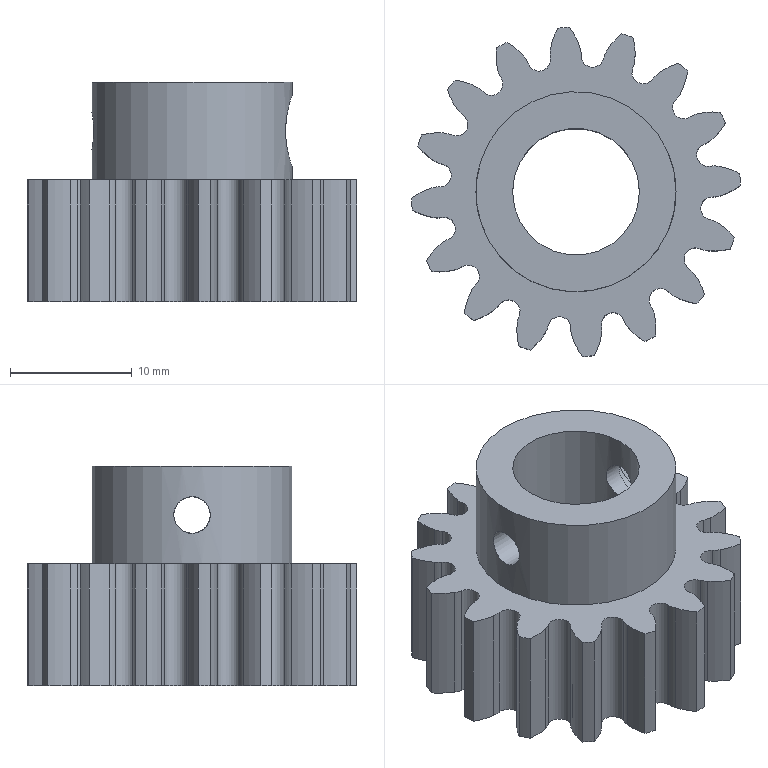Part | NX | features BREP 1, DATUM_CSYS 1 | 1 solid | 105 faces | box 26.979 x 26.979 x 18 mm | volume 4568 mm3 | cylinder 101 | plane 4 | commonest cylinder face diameters 4 x32 11.066 x32 1.87 x16 27 x16 3 x2 5.8 x1